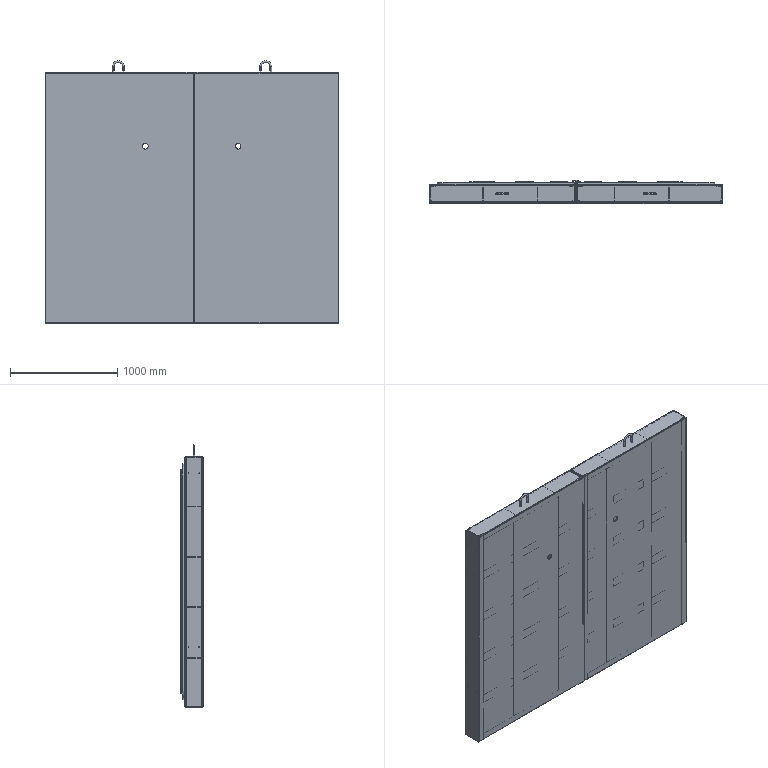Part | SolidWorks | features ReferencePattern 57, LocalLPattern 4, MirrorCompFeat 4 | 89 solids | 1441 faces | box 2740 x 211 x 2448 mm | volume 174205699 mm3 | plane 1145 | cylinder 260 | cone 24 | torus 12 | commonest cylinder face diameters 14 x96 8.5 x76 4 x20 6.8 x16 52 x12 13.835 x8